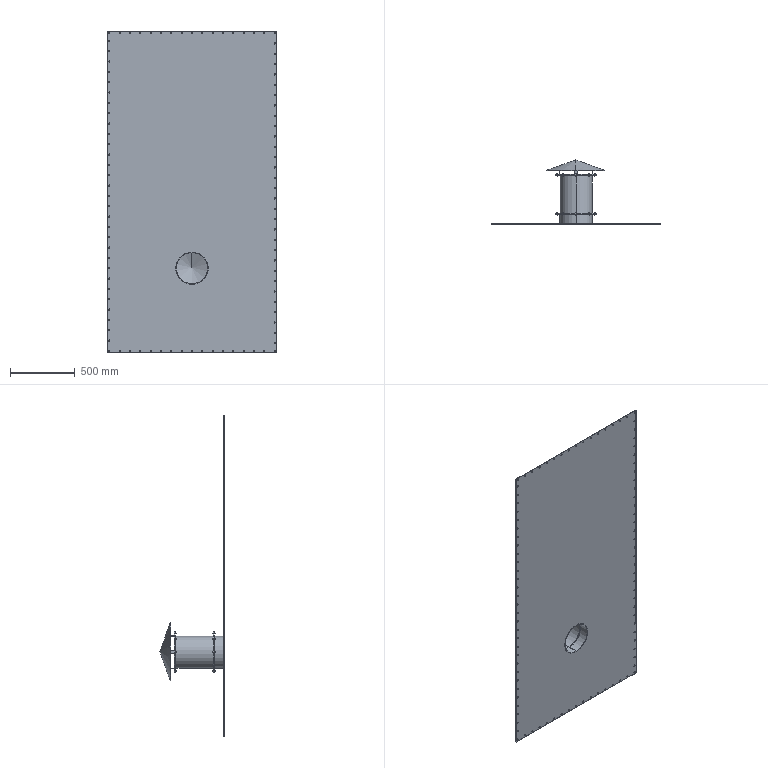Part | SolidWorks | features ReferencePattern 45, LocalCirPattern 1, LocalLPattern 1 | 60 solids | 1370 faces | box 1310 x 495.733 x 2490 mm | volume 15190258 mm3 | plane 478 | cylinder 470 | cone 390 | torus 32 | commonest cylinder face diameters 10 x188 4 x64 6 x64 4.1 x48 6.287 x48 7 x32